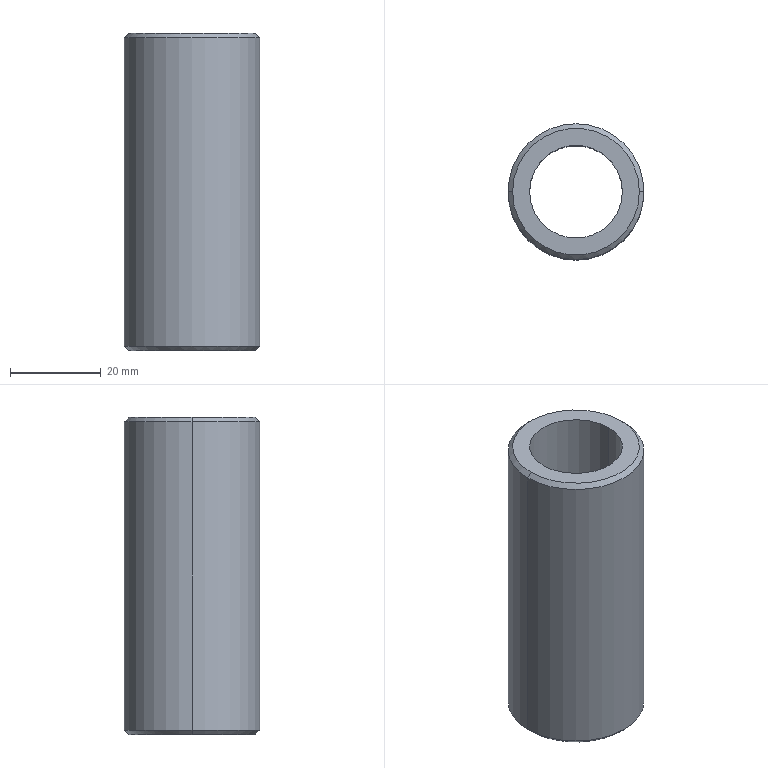Part | STEP file | Bushing_dia30_len75V11 | 1 solid | 10 faces | box 30 x 30 x 70 mm | volume 26283 mm3 | cone 4 | cylinder 4 | plane 2 | commonest cylinder face diameters 20.5 x2 30 x2
STEP:
#1=CARTESIAN_POINT('',(0.,0.,0.));
#2=DIRECTION('',(0.,0.,1.));
#3=DIRECTION('',(1.,0.,0.));
#4=AXIS2_PLACEMENT_3D('',#1,#2,#3);
#5=CARTESIAN_POINT('',(14.,0.,70.));
#6=VERTEX_POINT('',#5);
#7=CARTESIAN_POINT('',(-14.,0.,70.));
#8=VERTEX_POINT('',#7);
#9=CARTESIAN_POINT('',(0.,0.,70.));
#10=DIRECTION('',(0.,0.,1.));
#11=DIRECTION('',(1.,0.,0.));
#12=AXIS2_PLACEMENT_3D('',#9,#10,#11);
#13=CIRCLE('',#12,14.);
#14=CARTESIAN_POINT('',(0.,0.,70.));
#15=DIRECTION('',(0.,0.,-1.));
#16=DIRECTION('',(-1.,0.,0.));
#17=AXIS2_PLACEMENT_3D('',#14,#15,#16);
#18=CONICAL_SURFACE('',#17,14.,0.7854);
#19=CARTESIAN_POINT('',(3.142,0.));
#20=DIRECTION('',(-1.,0.));
#21=VECTOR('',#20,1.);
#22=LINE('',#19,#21);
#23=(GEOMETRIC_REPRESENTATION_CONTEXT(2)PARAMETRIC_REPRESENTATION_CONTEXT()REPRESENTATION_CONTEXT('',''));
#24=DEFINITIONAL_REPRESENTATION('',(#22),#23);
#25=PCURVE('',#18,#24);
#26=CARTESIAN_POINT('',(0.,0.,70.));
#27=DIRECTION('',(0.,0.,1.));
#28=DIRECTION('',(1.,0.,0.));
#29=AXIS2_PLACEMENT_3D('',#26,#27,#28);
#30=PLANE('',#29);
#31=CARTESIAN_POINT('',(0.,0.));
#32=DIRECTION('',(1.,0.));
#33=AXIS2_PLACEMENT_2D('',#31,#32);
#34=CIRCLE('',#33,14.);
#35=(GEOMETRIC_REPRESENTATION_CONTEXT(2)PARAMETRIC_REPRESENTATION_CONTEXT()REPRESENTATION_CONTEXT('',''));
#36=DEFINITIONAL_REPRESENTATION('',(#34),#35);
#37=PCURVE('',#30,#36);
#38=SURFACE_CURVE('',#13,(#25,#37),.PCURVE_S1.);
#39=EDGE_CURVE('',#6,#8,#38,.T.);
#40=ORIENTED_EDGE('',*,*,#39,.F.);
#41=CARTESIAN_POINT('',(15.,0.,69.));
#42=VERTEX_POINT('',#41);
#43=CARTESIAN_POINT('',(14.,0.,70.));
#44=DIRECTION('',(0.7071,0.,-0.7071));
#45=VECTOR('',#44,1.);
#46=LINE('',#43,#45);
#47=CARTESIAN_POINT('',(3.142,0.));
#48=DIRECTION('',(0.,1.));
#49=VECTOR('',#48,1.);
#50=LINE('',#47,#49);
#51=(GEOMETRIC_REPRESENTATION_CONTEXT(2)PARAMETRIC_REPRESENTATION_CONTEXT()REPRESENTATION_CONTEXT('',''));
#52=DEFINITIONAL_REPRESENTATION('',(#50),#51);
#53=PCURVE('',#18,#52);
#54=CARTESIAN_POINT('',(0.,0.,70.));
#55=DIRECTION('',(0.,0.,-1.));
#56=DIRECTION('',(-1.,0.,0.));
#57=AXIS2_PLACEMENT_3D('',#54,#55,#56);
#58=CONICAL_SURFACE('',#57,14.,0.7854);
#59=CARTESIAN_POINT('',(3.142,0.));
#60=DIRECTION('',(0.,1.));
#61=VECTOR('',#60,1.);
#62=LINE('',#59,#61);
#63=(GEOMETRIC_REPRESENTATION_CONTEXT(2)PARAMETRIC_REPRESENTATION_CONTEXT()REPRESENTATION_CONTEXT('',''));
#64=DEFINITIONAL_REPRESENTATION('',(#62),#63);
#65=PCURVE('',#58,#64);
#66=SURFACE_CURVE('',#46,(#53,#65),.PCURVE_S1.);
#67=EDGE_CURVE('',#6,#42,#66,.T.);
#68=ORIENTED_EDGE('',*,*,#67,.T.);
#69=CARTESIAN_POINT('',(-15.,0.,69.));
#70=VERTEX_POINT('',#69);
#71=CARTESIAN_POINT('',(0.,0.,69.));
#72=DIRECTION('',(0.,0.,-1.));
#73=DIRECTION('',(1.,0.,0.));
#74=AXIS2_PLACEMENT_3D('',#71,#72,#73);
#75=CIRCLE('',#74,15.);
#76=CARTESIAN_POINT('',(-3.142,1.));
#77=DIRECTION('',(1.,0.));
#78=VECTOR('',#77,1.);
#79=LINE('',#76,#78);
#80=(GEOMETRIC_REPRESENTATION_CONTEXT(2)PARAMETRIC_REPRESENTATION_CONTEXT()REPRESENTATION_CONTEXT('',''));
#81=DEFINITIONAL_REPRESENTATION('',(#79),#80);
#82=PCURVE('',#18,#81);
#83=CARTESIAN_POINT('',(0.,0.,70.));
#84=DIRECTION('',(0.,0.,-1.));
#85=DIRECTION('',(-1.,0.,0.));
#86=AXIS2_PLACEMENT_3D('',#83,#84,#85);
#87=CYLINDRICAL_SURFACE('',#86,15.);
#88=CARTESIAN_POINT('',(-3.142,1.));
#89=DIRECTION('',(1.,0.));
#90=VECTOR('',#89,1.);
#91=LINE('',#88,#90);
#92=(GEOMETRIC_REPRESENTATION_CONTEXT(2)PARAMETRIC_REPRESENTATION_CONTEXT()REPRESENTATION_CONTEXT('',''));
#93=DEFINITIONAL_REPRESENTATION('',(#91),#92);
#94=PCURVE('',#87,#93);
#95=SURFACE_CURVE('',#75,(#82,#94),.PCURVE_S1.);
#96=EDGE_CURVE('',#70,#42,#95,.T.);
#97=ORIENTED_EDGE('',*,*,#96,.F.);
#98=CARTESIAN_POINT('',(-14.,0.,70.));
#99=DIRECTION('',(-0.7071,0.,-0.7071));
#100=VECTOR('',#99,1.);
#101=LINE('',#98,#100);
#102=CARTESIAN_POINT('',(0.,0.));
#103=DIRECTION('',(0.,1.));
#104=VECTOR('',#103,1.);
#105=LINE('',#102,#104);
#106=(GEOMETRIC_REPRESENTATION_CONTEXT(2)PARAMETRIC_REPRESENTATION_CONTEXT()REPRESENTATION_CONTEXT('',''));
#107=DEFINITIONAL_REPRESENTATION('',(#105),#106);
#108=PCURVE('',#18,#107);
#109=CARTESIAN_POINT('',(6.283,0.));
#110=DIRECTION('',(0.,1.));
#111=VECTOR('',#110,1.);
#112=LINE('',#109,#111);
#113=(GEOMETRIC_REPRESENTATION_CONTEXT(2)PARAMETRIC_REPRESENTATION_CONTEXT()REPRESENTATION_CONTEXT('',''));
#114=DEFINITIONAL_REPRESENTATION('',(#112),#113);
#115=PCURVE('',#58,#114);
#116=SURFACE_CURVE('',#101,(#108,#115),.PCURVE_S1.);
#117=EDGE_CURVE('',#8,#70,#116,.T.);
#118=ORIENTED_EDGE('',*,*,#117,.F.);
#119=EDGE_LOOP('',(#40,#68,#97,#118));
#120=FACE_BOUND('',#119,.T.);
#121=ADVANCED_FACE('',(#120),#18,.T.);
#122=CARTESIAN_POINT('',(-14.,0.,0.));
#123=VERTEX_POINT('',#122);
#124=CARTESIAN_POINT('',(14.,0.,0.));
#125=VERTEX_POINT('',#124);
#126=CARTESIAN_POINT('',(0.,0.,0.));
#127=DIRECTION('',(0.,0.,-1.));
#128=DIRECTION('',(1.,0.,0.));
#129=AXIS2_PLACEMENT_3D('',#126,#127,#128);
#130=CIRCLE('',#129,14.);
#131=CARTESIAN_POINT('',(0.,0.,1.));
#132=DIRECTION('',(0.,0.,1.));
#133=DIRECTION('',(1.,0.,0.));
#134=AXIS2_PLACEMENT_3D('',#131,#132,#133);
#135=CONICAL_SURFACE('',#134,15.,0.7854);
#136=CARTESIAN_POINT('',(6.283,-1.));
#137=DIRECTION('',(-1.,0.));
#138=VECTOR('',#137,1.);
#139=LINE('',#136,#138);
#140=(GEOMETRIC_REPRESENTATION_CONTEXT(2)PARAMETRIC_REPRESENTATION_CONTEXT()REPRESENTATION_CONTEXT('',''));
#141=DEFINITIONAL_REPRESENTATION('',(#139),#140);
#142=PCURVE('',#135,#141);
#143=CARTESIAN_POINT('',(0.,0.,0.));
#144=DIRECTION('',(0.,0.,1.));
#145=DIRECTION('',(1.,0.,0.));
#146=AXIS2_PLACEMENT_3D('',#143,#144,#145);
#147=PLANE('',#146);
#148=CARTESIAN_POINT('',(14.,0.));
#149=CARTESIAN_POINT('',(14.,-24.249));
#150=CARTESIAN_POINT('',(-7.,-12.124));
#151=CARTESIAN_POINT('',(-28.,0.));
#152=CARTESIAN_POINT('',(-7.,12.124));
#153=CARTESIAN_POINT('',(14.,24.249));
#154=CARTESIAN_POINT('',(14.,0.));
#155=(BOUNDED_CURVE()B_SPLINE_CURVE(2,(#148,#149,#150,#151,#152,#153,#154),.UNSPECIFIED.,.T.,.F.)B_SPLINE_CURVE_WITH_KNOTS((1,2,2,2,2,1),(-2.094,0.,2.094,4.189,6.283,8.378),.UNSPECIFIED.)CURVE()GEOMETRIC_REPRESENTATION_ITEM()RATIONAL_B_SPLINE_CURVE((1.,0.5,1.,0.5,1.,0.5,1.))REPRESENTATION_ITEM(''));
#156=(GEOMETRIC_REPRESENTATION_CONTEXT(2)PARAMETRIC_REPRESENTATION_CONTEXT()REPRESENTATION_CONTEXT('',''));
#157=DEFINITIONAL_REPRESENTATION('',(#155),#156);
#158=PCURVE('',#147,#157);
#159=SURFACE_CURVE('',#130,(#142,#158),.PCURVE_S1.);
#160=EDGE_CURVE('',#123,#125,#159,.T.);
#161=ORIENTED_EDGE('',*,*,#160,.F.);
#162=CARTESIAN_POINT('',(-15.,0.,1.));
#163=VERTEX_POINT('',#162);
#164=CARTESIAN_POINT('',(-15.,0.,1.));
#165=DIRECTION('',(-0.7071,0.,0.7071));
#166=VECTOR('',#165,1.);
#167=LINE('',#164,#166);
#168=CARTESIAN_POINT('',(3.142,0.));
#169=DIRECTION('',(0.,1.));
#170=VECTOR('',#169,1.);
#171=LINE('',#168,#170);
#172=(GEOMETRIC_REPRESENTATION_CONTEXT(2)PARAMETRIC_REPRESENTATION_CONTEXT()REPRESENTATION_CONTEXT('',''));
#173=DEFINITIONAL_REPRESENTATION('',(#171),#172);
#174=PCURVE('',#135,#173);
#175=CARTESIAN_POINT('',(0.,0.,1.));
#176=DIRECTION('',(0.,0.,1.));
#177=DIRECTION('',(1.,0.,0.));
#178=AXIS2_PLACEMENT_3D('',#175,#176,#177);
#179=CONICAL_SURFACE('',#178,15.,0.7854);
#180=CARTESIAN_POINT('',(3.142,0.));
#181=DIRECTION('',(0.,1.));
#182=VECTOR('',#181,1.);
#183=LINE('',#180,#182);
#184=(GEOMETRIC_REPRESENTATION_CONTEXT(2)PARAMETRIC_REPRESENTATION_CONTEXT()REPRESENTATION_CONTEXT('',''));
#185=DEFINITIONAL_REPRESENTATION('',(#183),#184);
#186=PCURVE('',#179,#185);
#187=SURFACE_CURVE('',#167,(#174,#186),.PCURVE_S1.);
#188=EDGE_CURVE('',#123,#163,#187,.T.);
#189=ORIENTED_EDGE('',*,*,#188,.T.);
#190=CARTESIAN_POINT('',(15.,0.,1.));
#191=VERTEX_POINT('',#190);
#192=CARTESIAN_POINT('',(0.,0.,1.));
#193=DIRECTION('',(0.,0.,1.));
#194=DIRECTION('',(1.,0.,0.));
#195=AXIS2_PLACEMENT_3D('',#192,#193,#194);
#196=CIRCLE('',#195,15.);
#197=CARTESIAN_POINT('',(0.,0.));
#198=DIRECTION('',(1.,0.));
#199=VECTOR('',#198,1.);
#200=LINE('',#197,#199);
#201=(GEOMETRIC_REPRESENTATION_CONTEXT(2)PARAMETRIC_REPRESENTATION_CONTEXT()REPRESENTATION_CONTEXT('',''));
#202=DEFINITIONAL_REPRESENTATION('',(#200),#201);
#203=PCURVE('',#135,#202);
#204=CARTESIAN_POINT('',(3.142,69.));
#205=DIRECTION('',(-1.,0.));
#206=VECTOR('',#205,1.);
#207=LINE('',#204,#206);
#208=(GEOMETRIC_REPRESENTATION_CONTEXT(2)PARAMETRIC_REPRESENTATION_CONTEXT()REPRESENTATION_CONTEXT('',''));
#209=DEFINITIONAL_REPRESENTATION('',(#207),#208);
#210=PCURVE('',#87,#209);
#211=SURFACE_CURVE('',#196,(#203,#210),.PCURVE_S1.);
#212=EDGE_CURVE('',#191,#163,#211,.T.);
#213=ORIENTED_EDGE('',*,*,#212,.F.);
#214=CARTESIAN_POINT('',(15.,0.,1.));
#215=DIRECTION('',(0.7071,0.,0.7071));
#216=VECTOR('',#215,1.);
#217=LINE('',#214,#216);
#218=CARTESIAN_POINT('',(0.,0.));
#219=DIRECTION('',(0.,1.));
#220=VECTOR('',#219,1.);
#221=LINE('',#218,#220);
#222=(GEOMETRIC_REPRESENTATION_CONTEXT(2)PARAMETRIC_REPRESENTATION_CONTEXT()REPRESENTATION_CONTEXT('',''));
#223=DEFINITIONAL_REPRESENTATION('',(#221),#222);
#224=PCURVE('',#135,#223);
#225=CARTESIAN_POINT('',(6.283,0.));
#226=DIRECTION('',(0.,1.));
#227=VECTOR('',#226,1.);
#228=LINE('',#225,#227);
#229=(GEOMETRIC_REPRESENTATION_CONTEXT(2)PARAMETRIC_REPRESENTATION_CONTEXT()REPRESENTATION_CONTEXT('',''));
#230=DEFINITIONAL_REPRESENTATION('',(#228),#229);
#231=PCURVE('',#179,#230);
#232=SURFACE_CURVE('',#217,(#224,#231),.PCURVE_S1.);
#233=EDGE_CURVE('',#125,#191,#232,.T.);
#234=ORIENTED_EDGE('',*,*,#233,.F.);
#235=EDGE_LOOP('',(#161,#189,#213,#234));
#236=FACE_BOUND('',#235,.T.);
#237=ADVANCED_FACE('',(#236),#135,.T.);
#238=CARTESIAN_POINT('',(-10.25,0.,70.));
#239=VERTEX_POINT('',#238);
#240=CARTESIAN_POINT('',(-10.25,0.,0.));
#241=VERTEX_POINT('',#240);
#242=CARTESIAN_POINT('',(-10.25,0.,70.));
#243=DIRECTION('',(0.,0.,-1.));
#244=VECTOR('',#243,1.);
#245=LINE('',#242,#244);
#246=CARTESIAN_POINT('',(0.,0.,70.));
#247=DIRECTION('',(0.,0.,-1.));
#248=DIRECTION('',(-1.,0.,0.));
#249=AXIS2_PLACEMENT_3D('',#246,#247,#248);
#250=CYLINDRICAL_SURFACE('',#249,10.25);
#251=CARTESIAN_POINT('',(6.283,0.));
#252=DIRECTION('',(0.,1.));
#253=VECTOR('',#252,1.);
#254=LINE('',#251,#253);
#255=(GEOMETRIC_REPRESENTATION_CONTEXT(2)PARAMETRIC_REPRESENTATION_CONTEXT()REPRESENTATION_CONTEXT('',''));
#256=DEFINITIONAL_REPRESENTATION('',(#254),#255);
#257=PCURVE('',#250,#256);
#258=CARTESIAN_POINT('',(0.,0.,70.));
#259=DIRECTION('',(0.,0.,-1.));
#260=DIRECTION('',(-1.,0.,0.));
#261=AXIS2_PLACEMENT_3D('',#258,#259,#260);
#262=CYLINDRICAL_SURFACE('',#261,10.25);
#263=CARTESIAN_POINT('',(0.,0.));
#264=DIRECTION('',(0.,1.));
#265=VECTOR('',#264,1.);
#266=LINE('',#263,#265);
#267=(GEOMETRIC_REPRESENTATION_CONTEXT(2)PARAMETRIC_REPRESENTATION_CONTEXT()REPRESENTATION_CONTEXT('',''));
#268=DEFINITIONAL_REPRESENTATION('',(#266),#267);
#269=PCURVE('',#262,#268);
#270=SURFACE_CURVE('',#245,(#257,#269),.PCURVE_S1.);
#271=EDGE_CURVE('',#239,#241,#270,.T.);
#272=ORIENTED_EDGE('',*,*,#271,.T.);
#273=CARTESIAN_POINT('',(10.25,0.,0.));
#274=VERTEX_POINT('',#273);
#275=CARTESIAN_POINT('',(0.,0.,0.));
#276=DIRECTION('',(0.,0.,1.));
#277=DIRECTION('',(1.,0.,0.));
#278=AXIS2_PLACEMENT_3D('',#275,#276,#277);
#279=CIRCLE('',#278,10.25);
#280=CARTESIAN_POINT('',(9.425,70.));
#281=DIRECTION('',(-1.,0.));
#282=VECTOR('',#281,1.);
#283=LINE('',#280,#282);
#284=(GEOMETRIC_REPRESENTATION_CONTEXT(2)PARAMETRIC_REPRESENTATION_CONTEXT()REPRESENTATION_CONTEXT('',''));
#285=DEFINITIONAL_REPRESENTATION('',(#283),#284);
#286=PCURVE('',#250,#285);
#287=CARTESIAN_POINT('',(0.,0.));
#288=DIRECTION('',(1.,0.));
#289=AXIS2_PLACEMENT_2D('',#287,#288);
#290=CIRCLE('',#289,10.25);
#291=(GEOMETRIC_REPRESENTATION_CONTEXT(2)PARAMETRIC_REPRESENTATION_CONTEXT()REPRESENTATION_CONTEXT('',''));
#292=DEFINITIONAL_REPRESENTATION('',(#290),#291);
#293=PCURVE('',#147,#292);
#294=SURFACE_CURVE('',#279,(#286,#293),.PCURVE_S1.);
#295=EDGE_CURVE('',#241,#274,#294,.T.);
#296=ORIENTED_EDGE('',*,*,#295,.T.);
#297=CARTESIAN_POINT('',(10.25,0.,70.));
#298=VERTEX_POINT('',#297);
#299=CARTESIAN_POINT('',(10.25,0.,70.));
#300=DIRECTION('',(0.,0.,-1.));
#301=VECTOR('',#300,1.);
#302=LINE('',#299,#301);
#303=CARTESIAN_POINT('',(3.142,0.));
#304=DIRECTION('',(0.,1.));
#305=VECTOR('',#304,1.);
#306=LINE('',#303,#305);
#307=(GEOMETRIC_REPRESENTATION_CONTEXT(2)PARAMETRIC_REPRESENTATION_CONTEXT()REPRESENTATION_CONTEXT('',''));
#308=DEFINITIONAL_REPRESENTATION('',(#306),#307);
#309=PCURVE('',#250,#308);
#310=CARTESIAN_POINT('',(3.142,0.));
#311=DIRECTION('',(0.,1.));
#312=VECTOR('',#311,1.);
#313=LINE('',#310,#312);
#314=(GEOMETRIC_REPRESENTATION_CONTEXT(2)PARAMETRIC_REPRESENTATION_CONTEXT()REPRESENTATION_CONTEXT('',''));
#315=DEFINITIONAL_REPRESENTATION('',(#313),#314);
#316=PCURVE('',#262,#315);
#317=SURFACE_CURVE('',#302,(#309,#316),.PCURVE_S1.);
#318=EDGE_CURVE('',#298,#274,#317,.T.);
#319=ORIENTED_EDGE('',*,*,#318,.F.);
#320=CARTESIAN_POINT('',(0.,0.,70.));
#321=DIRECTION('',(0.,0.,1.));
#322=DIRECTION('',(1.,0.,0.));
#323=AXIS2_PLACEMENT_3D('',#320,#321,#322);
#324=CIRCLE('',#323,10.25);
#325=CARTESIAN_POINT('',(9.425,0.));
#326=DIRECTION('',(-1.,0.));
#327=VECTOR('',#326,1.);
#328=LINE('',#325,#327);
#329=(GEOMETRIC_REPRESENTATION_CONTEXT(2)PARAMETRIC_REPRESENTATION_CONTEXT()REPRESENTATION_CONTEXT('',''));
#330=DEFINITIONAL_REPRESENTATION('',(#328),#329);
#331=PCURVE('',#250,#330);
#332=CARTESIAN_POINT('',(0.,0.));
#333=DIRECTION('',(1.,0.));
#334=AXIS2_PLACEMENT_2D('',#332,#333);
#335=CIRCLE('',#334,10.25);
#336=(GEOMETRIC_REPRESENTATION_CONTEXT(2)PARAMETRIC_REPRESENTATION_CONTEXT()REPRESENTATION_CONTEXT('',''));
#337=DEFINITIONAL_REPRESENTATION('',(#335),#336);
#338=PCURVE('',#30,#337);
#339=SURFACE_CURVE('',#324,(#331,#338),.PCURVE_S1.);
#340=EDGE_CURVE('',#239,#298,#339,.T.);
#341=ORIENTED_EDGE('',*,*,#340,.F.);
#342=EDGE_LOOP('',(#272,#296,#319,#341));
#343=FACE_BOUND('',#342,.F.);
#344=ADVANCED_FACE('',(#343),#250,.F.);
#345=ORIENTED_EDGE('',*,*,#96,.T.);
#346=CARTESIAN_POINT('',(15.,0.,70.));
#347=DIRECTION('',(0.,0.,-1.));
#348=VECTOR('',#347,1.);
#349=LINE('',#346,#348);
#350=CARTESIAN_POINT('',(3.142,0.));
#351=DIRECTION('',(0.,1.));
#352=VECTOR('',#351,1.);
#353=LINE('',#350,#352);
#354=(GEOMETRIC_REPRESENTATION_CONTEXT(2)PARAMETRIC_REPRESENTATION_CONTEXT()REPRESENTATION_CONTEXT('',''));
#355=DEFINITIONAL_REPRESENTATION('',(#353),#354);
#356=PCURVE('',#87,#355);
#357=CARTESIAN_POINT('',(0.,0.,70.));
#358=DIRECTION('',(0.,0.,-1.));
#359=DIRECTION('',(-1.,0.,0.));
#360=AXIS2_PLACEMENT_3D('',#357,#358,#359);
#361=CYLINDRICAL_SURFACE('',#360,15.);
#362=CARTESIAN_POINT('',(3.142,0.));
#363=DIRECTION('',(0.,1.));
#364=VECTOR('',#363,1.);
#365=LINE('',#362,#364);
#366=(GEOMETRIC_REPRESENTATION_CONTEXT(2)PARAMETRIC_REPRESENTATION_CONTEXT()REPRESENTATION_CONTEXT('',''));
#367=DEFINITIONAL_REPRESENTATION('',(#365),#366);
#368=PCURVE('',#361,#367);
#369=SURFACE_CURVE('',#349,(#356,#368),.PCURVE_S1.);
#370=EDGE_CURVE('',#42,#191,#369,.T.);
#371=ORIENTED_EDGE('',*,*,#370,.T.);
#372=ORIENTED_EDGE('',*,*,#212,.T.);
#373=CARTESIAN_POINT('',(-15.,0.,70.));
#374=DIRECTION('',(0.,0.,-1.));
#375=VECTOR('',#374,1.);
#376=LINE('',#373,#375);
#377=CARTESIAN_POINT('',(0.,0.));
#378=DIRECTION('',(0.,1.));
#379=VECTOR('',#378,1.);
#380=LINE('',#377,#379);
#381=(GEOMETRIC_REPRESENTATION_CONTEXT(2)PARAMETRIC_REPRESENTATION_CONTEXT()REPRESENTATION_CONTEXT('',''));
#382=DEFINITIONAL_REPRESENTATION('',(#380),#381);
#383=PCURVE('',#87,#382);
#384=CARTESIAN_POINT('',(6.283,0.));
#385=DIRECTION('',(0.,1.));
#386=VECTOR('',#385,1.);
#387=LINE('',#384,#386);
#388=(GEOMETRIC_REPRESENTATION_CONTEXT(2)PARAMETRIC_REPRESENTATION_CONTEXT()REPRESENTATION_CONTEXT('',''));
#389=DEFINITIONAL_REPRESENTATION('',(#387),#388);
#390=PCURVE('',#361,#389);
#391=SURFACE_CURVE('',#376,(#383,#390),.PCURVE_S1.);
#392=EDGE_CURVE('',#70,#163,#391,.T.);
#393=ORIENTED_EDGE('',*,*,#392,.F.);
#394=EDGE_LOOP('',(#345,#371,#372,#393));
#395=FACE_BOUND('',#394,.T.);
#396=ADVANCED_FACE('',(#395),#87,.T.);
#397=CARTESIAN_POINT('',(0.,0.,70.));
#398=DIRECTION('',(0.,0.,1.));
#399=DIRECTION('',(1.,0.,0.));
#400=AXIS2_PLACEMENT_3D('',#397,#398,#399);
#401=CIRCLE('',#400,14.);
#402=CARTESIAN_POINT('',(0.,0.));
#403=DIRECTION('',(1.,0.));
#404=AXIS2_PLACEMENT_2D('',#402,#403);
#405=CIRCLE('',#404,14.);
#406=(GEOMETRIC_REPRESENTATION_CONTEXT(2)PARAMETRIC_REPRESENTATION_CONTEXT()REPRESENTATION_CONTEXT('',''));
#407=DEFINITIONAL_REPRESENTATION('',(#405),#406);
#408=PCURVE('',#30,#407);
#409=CARTESIAN_POINT('',(9.425,0.));
#410=DIRECTION('',(-1.,0.));
#411=VECTOR('',#410,1.);
#412=LINE('',#409,#411);
#413=(GEOMETRIC_REPRESENTATION_CONTEXT(2)PARAMETRIC_REPRESENTATION_CONTEXT()REPRESENTATION_CONTEXT('',''));
#414=DEFINITIONAL_REPRESENTATION('',(#412),#413);
#415=PCURVE('',#58,#414);
#416=SURFACE_CURVE('',#401,(#408,#415),.PCURVE_S1.);
#417=EDGE_CURVE('',#8,#6,#416,.T.);
#418=ORIENTED_EDGE('',*,*,#417,.T.);
#419=ORIENTED_EDGE('',*,*,#39,.T.);
#420=EDGE_LOOP('',(#418,#419));
#421=FACE_BOUND('',#420,.T.);
#422=ORIENTED_EDGE('',*,*,#340,.F.);
#423=CARTESIAN_POINT('',(0.,0.,70.));
#424=DIRECTION('',(0.,0.,1.));
#425=DIRECTION('',(1.,0.,0.));
#426=AXIS2_PLACEMENT_3D('',#423,#424,#425);
#427=CIRCLE('',#426,10.25);
#428=CARTESIAN_POINT('',(0.,0.));
#429=DIRECTION('',(1.,0.));
#430=AXIS2_PLACEMENT_2D('',#428,#429);
#431=CIRCLE('',#430,10.25);
#432=(GEOMETRIC_REPRESENTATION_CONTEXT(2)PARAMETRIC_REPRESENTATION_CONTEXT()REPRESENTATION_CONTEXT('',''));
#433=DEFINITIONAL_REPRESENTATION('',(#431),#432);
#434=PCURVE('',#30,#433);
#435=CARTESIAN_POINT('',(3.142,0.));
#436=DIRECTION('',(-1.,0.));
#437=VECTOR('',#436,1.);
#438=LINE('',#435,#437);
#439=(GEOMETRIC_REPRESENTATION_CONTEXT(2)PARAMETRIC_REPRESENTATION_CONTEXT()REPRESENTATION_CONTEXT('',''));
#440=DEFINITIONAL_REPRESENTATION('',(#438),#439);
#441=PCURVE('',#262,#440);
#442=SURFACE_CURVE('',#427,(#434,#441),.PCURVE_S1.);
#443=EDGE_CURVE('',#298,#239,#442,.T.);
#444=ORIENTED_EDGE('',*,*,#443,.F.);
#445=EDGE_LOOP('',(#422,#444));
#446=FACE_BOUND('',#445,.T.);
#447=ADVANCED_FACE('',(#421,#446),#30,.T.);
#448=CARTESIAN_POINT('',(0.,0.,0.));
#449=DIRECTION('',(0.,0.,-1.));
#450=DIRECTION('',(1.,0.,0.));
#451=AXIS2_PLACEMENT_3D('',#448,#449,#450);
#452=CIRCLE('',#451,14.);
#453=CARTESIAN_POINT('',(14.,0.));
#454=CARTESIAN_POINT('',(14.,-24.249));
#455=CARTESIAN_POINT('',(-7.,-12.124));
#456=CARTESIAN_POINT('',(-28.,0.));
#457=CARTESIAN_POINT('',(-7.,12.124));
#458=CARTESIAN_POINT('',(14.,24.249));
#459=CARTESIAN_POINT('',(14.,0.));
#460=(BOUNDED_CURVE()B_SPLINE_CURVE(2,(#453,#454,#455,#456,#457,#458,#459),.UNSPECIFIED.,.T.,.F.)B_SPLINE_CURVE_WITH_KNOTS((1,2,2,2,2,1),(-2.094,0.,2.094,4.189,6.283,8.378),.UNSPECIFIED.)CURVE()GEOMETRIC_REPRESENTATION_ITEM()RATIONAL_B_SPLINE_CURVE((1.,0.5,1.,0.5,1.,0.5,1.))REPRESENTATION_ITEM(''));
#461=(GEOMETRIC_REPRESENTATION_CONTEXT(2)PARAMETRIC_REPRESENTATION_CONTEXT()REPRESENTATION_CONTEXT('',''));
#462=DEFINITIONAL_REPRESENTATION('',(#460),#461);
#463=PCURVE('',#147,#462);
#464=CARTESIAN_POINT('',(6.283,-1.));
#465=DIRECTION('',(-1.,0.));
#466=VECTOR('',#465,1.);
#467=LINE('',#464,#466);
#468=(GEOMETRIC_REPRESENTATION_CONTEXT(2)PARAMETRIC_REPRESENTATION_CONTEXT()REPRESENTATION_CONTEXT('',''));
#469=DEFINITIONAL_REPRESENTATION('',(#467),#468);
#470=PCURVE('',#179,#469);
#471=SURFACE_CURVE('',#452,(#463,#470),.PCURVE_S1.);
#472=EDGE_CURVE('',#125,#123,#471,.T.);
#473=ORIENTED_EDGE('',*,*,#472,.T.);
#474=ORIENTED_EDGE('',*,*,#160,.T.);
#475=EDGE_LOOP('',(#473,#474));
#476=FACE_BOUND('',#475,.T.);
#477=ORIENTED_EDGE('',*,*,#295,.T.);
#478=CARTESIAN_POINT('',(0.,0.,0.));
#479=DIRECTION('',(0.,0.,1.));
#480=DIRECTION('',(1.,0.,0.));
#481=AXIS2_PLACEMENT_3D('',#478,#479,#480);
#482=CIRCLE('',#481,10.25);
#483=CARTESIAN_POINT('',(0.,0.));
#484=DIRECTION('',(1.,0.));
#485=AXIS2_PLACEMENT_2D('',#483,#484);
#486=CIRCLE('',#485,10.25);
#487=(GEOMETRIC_REPRESENTATION_CONTEXT(2)PARAMETRIC_REPRESENTATION_CONTEXT()REPRESENTATION_CONTEXT('',''));
#488=DEFINITIONAL_REPRESENTATION('',(#486),#487);
#489=PCURVE('',#147,#488);
#490=CARTESIAN_POINT('',(3.142,70.));
#491=DIRECTION('',(-1.,0.));
#492=VECTOR('',#491,1.);
#493=LINE('',#490,#492);
#494=(GEOMETRIC_REPRESENTATION_CONTEXT(2)PARAMETRIC_REPRESENTATION_CONTEXT()REPRESENTATION_CONTEXT('',''));
#495=DEFINITIONAL_REPRESENTATION('',(#493),#494);
#496=PCURVE('',#262,#495);
#497=SURFACE_CURVE('',#482,(#489,#496),.PCURVE_S1.);
#498=EDGE_CURVE('',#274,#241,#497,.T.);
#499=ORIENTED_EDGE('',*,*,#498,.T.);
#500=EDGE_LOOP('',(#477,#499));
#501=FACE_BOUND('',#500,.T.);
#502=ADVANCED_FACE('',(#476,#501),#147,.F.);
#503=ORIENTED_EDGE('',*,*,#370,.F.);
#504=CARTESIAN_POINT('',(0.,0.,69.));
#505=DIRECTION('',(0.,0.,-1.));
#506=DIRECTION('',(1.,0.,0.));
#507=AXIS2_PLACEMENT_3D('',#504,#505,#506);
#508=CIRCLE('',#507,15.);
#509=CARTESIAN_POINT('',(3.142,1.));
#510=DIRECTION('',(1.,0.));
#511=VECTOR('',#510,1.);
#512=LINE('',#509,#511);
#513=(GEOMETRIC_REPRESENTATION_CONTEXT(2)PARAMETRIC_REPRESENTATION_CONTEXT()REPRESENTATION_CONTEXT('',''));
#514=DEFINITIONAL_REPRESENTATION('',(#512),#513);
#515=PCURVE('',#361,#514);
#516=CARTESIAN_POINT('',(3.142,1.));
#517=DIRECTION('',(1.,0.));
#518=VECTOR('',#517,1.);
#519=LINE('',#516,#518);
#520=(GEOMETRIC_REPRESENTATION_CONTEXT(2)PARAMETRIC_REPRESENTATION_CONTEXT()REPRESENTATION_CONTEXT('',''));
#521=DEFINITIONAL_REPRESENTATION('',(#519),#520);
#522=PCURVE('',#58,#521);
#523=SURFACE_CURVE('',#508,(#515,#522),.PCURVE_S1.);
#524=EDGE_CURVE('',#42,#70,#523,.T.);
#525=ORIENTED_EDGE('',*,*,#524,.T.);
#526=ORIENTED_EDGE('',*,*,#392,.T.);
#527=CARTESIAN_POINT('',(0.,0.,1.));
#528=DIRECTION('',(0.,0.,1.));
#529=DIRECTION('',(1.,0.,0.));
#530=AXIS2_PLACEMENT_3D('',#527,#528,#529);
#531=CIRCLE('',#530,15.);
#532=CARTESIAN_POINT('',(9.425,69.));
#533=DIRECTION('',(-1.,0.));
#534=VECTOR('',#533,1.);
#535=LINE('',#532,#534);
#536=(GEOMETRIC_REPRESENTATION_CONTEXT(2)PARAMETRIC_REPRESENTATION_CONTEXT()REPRESENTATION_CONTEXT('',''));
#537=DEFINITIONAL_REPRESENTATION('',(#535),#536);
#538=PCURVE('',#361,#537);
#539=CARTESIAN_POINT('',(0.,0.));
#540=DIRECTION('',(1.,0.));
#541=VECTOR('',#540,1.);
#542=LINE('',#539,#541);
#543=(GEOMETRIC_REPRESENTATION_CONTEXT(2)PARAMETRIC_REPRESENTATION_CONTEXT()REPRESENTATION_CONTEXT('',''));
#544=DEFINITIONAL_REPRESENTATION('',(#542),#543);
#545=PCURVE('',#179,#544);
#546=SURFACE_CURVE('',#531,(#538,#545),.PCURVE_S1.);
#547=EDGE_CURVE('',#163,#191,#546,.T.);
#548=ORIENTED_EDGE('',*,*,#547,.T.);
#549=EDGE_LOOP('',(#503,#525,#526,#548));
#550=FACE_BOUND('',#549,.T.);
#551=ADVANCED_FACE('',(#550),#361,.T.);
#552=ORIENTED_EDGE('',*,*,#498,.T.);
#553=ORIENTED_EDGE('',*,*,#271,.F.);
#554=ORIENTED_EDGE('',*,*,#443,.F.);
#555=ORIENTED_EDGE('',*,*,#318,.T.);
#556=EDGE_LOOP('',(#552,#553,#554,#555));
#557=FACE_BOUND('',#556,.F.);
#558=ADVANCED_FACE('',(#557),#262,.F.);
#559=ORIENTED_EDGE('',*,*,#188,.F.);
#560=ORIENTED_EDGE('',*,*,#472,.F.);
#561=ORIENTED_EDGE('',*,*,#233,.T.);
#562=ORIENTED_EDGE('',*,*,#547,.F.);
#563=EDGE_LOOP('',(#559,#560,#561,#562));
#564=FACE_BOUND('',#563,.T.);
#565=ADVANCED_FACE('',(#564),#179,.T.);
#566=ORIENTED_EDGE('',*,*,#67,.F.);
#567=ORIENTED_EDGE('',*,*,#417,.F.);
#568=ORIENTED_EDGE('',*,*,#117,.T.);
#569=ORIENTED_EDGE('',*,*,#524,.F.);
#570=EDGE_LOOP('',(#566,#567,#568,#569));
#571=FACE_BOUND('',#570,.T.);
#572=ADVANCED_FACE('',(#571),#58,.T.);
#573=CLOSED_SHELL('',(#121,#237,#344,#396,#447,#502,#551,#558,#565,#572));
#574=MANIFOLD_SOLID_BREP('',#573);
#575=(LENGTH_UNIT()NAMED_UNIT(*)SI_UNIT(.MILLI.,.METRE.));
#576=UNCERTAINTY_MEASURE_WITH_UNIT(LENGTH_MEASURE(0.0000001),#575,'','');
#577=(NAMED_UNIT(*)PLANE_ANGLE_UNIT()SI_UNIT($,.RADIAN.));
#578=(NAMED_UNIT(*)SI_UNIT($,.STERADIAN.)SOLID_ANGLE_UNIT());
#579=(GEOMETRIC_REPRESENTATION_CONTEXT(3)GLOBAL_UNCERTAINTY_ASSIGNED_CONTEXT((#576))GLOBAL_UNIT_ASSIGNED_CONTEXT((#575,#577,#578))REPRESENTATION_CONTEXT('',''));
#580=ADVANCED_BREP_SHAPE_REPRESENTATION('',(#4,#574),#579);